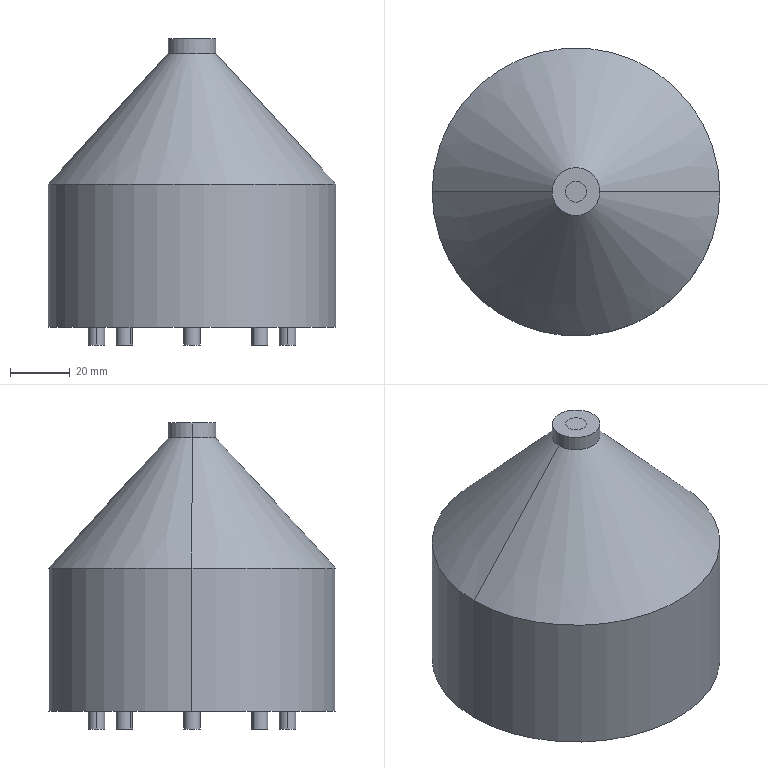Part | STEP file | LPFD27003500MHz_step | 10 solids | 169 faces | box 96.34 x 96.34 x 102.43 mm | volume 664889 mm3 | cylinder 110 | plane 55 | cone 4 | commonest cylinder face diameters 1.6 x32 5.5 x32 2.4 x16 3.2 x16 7 x4 8.9 x2